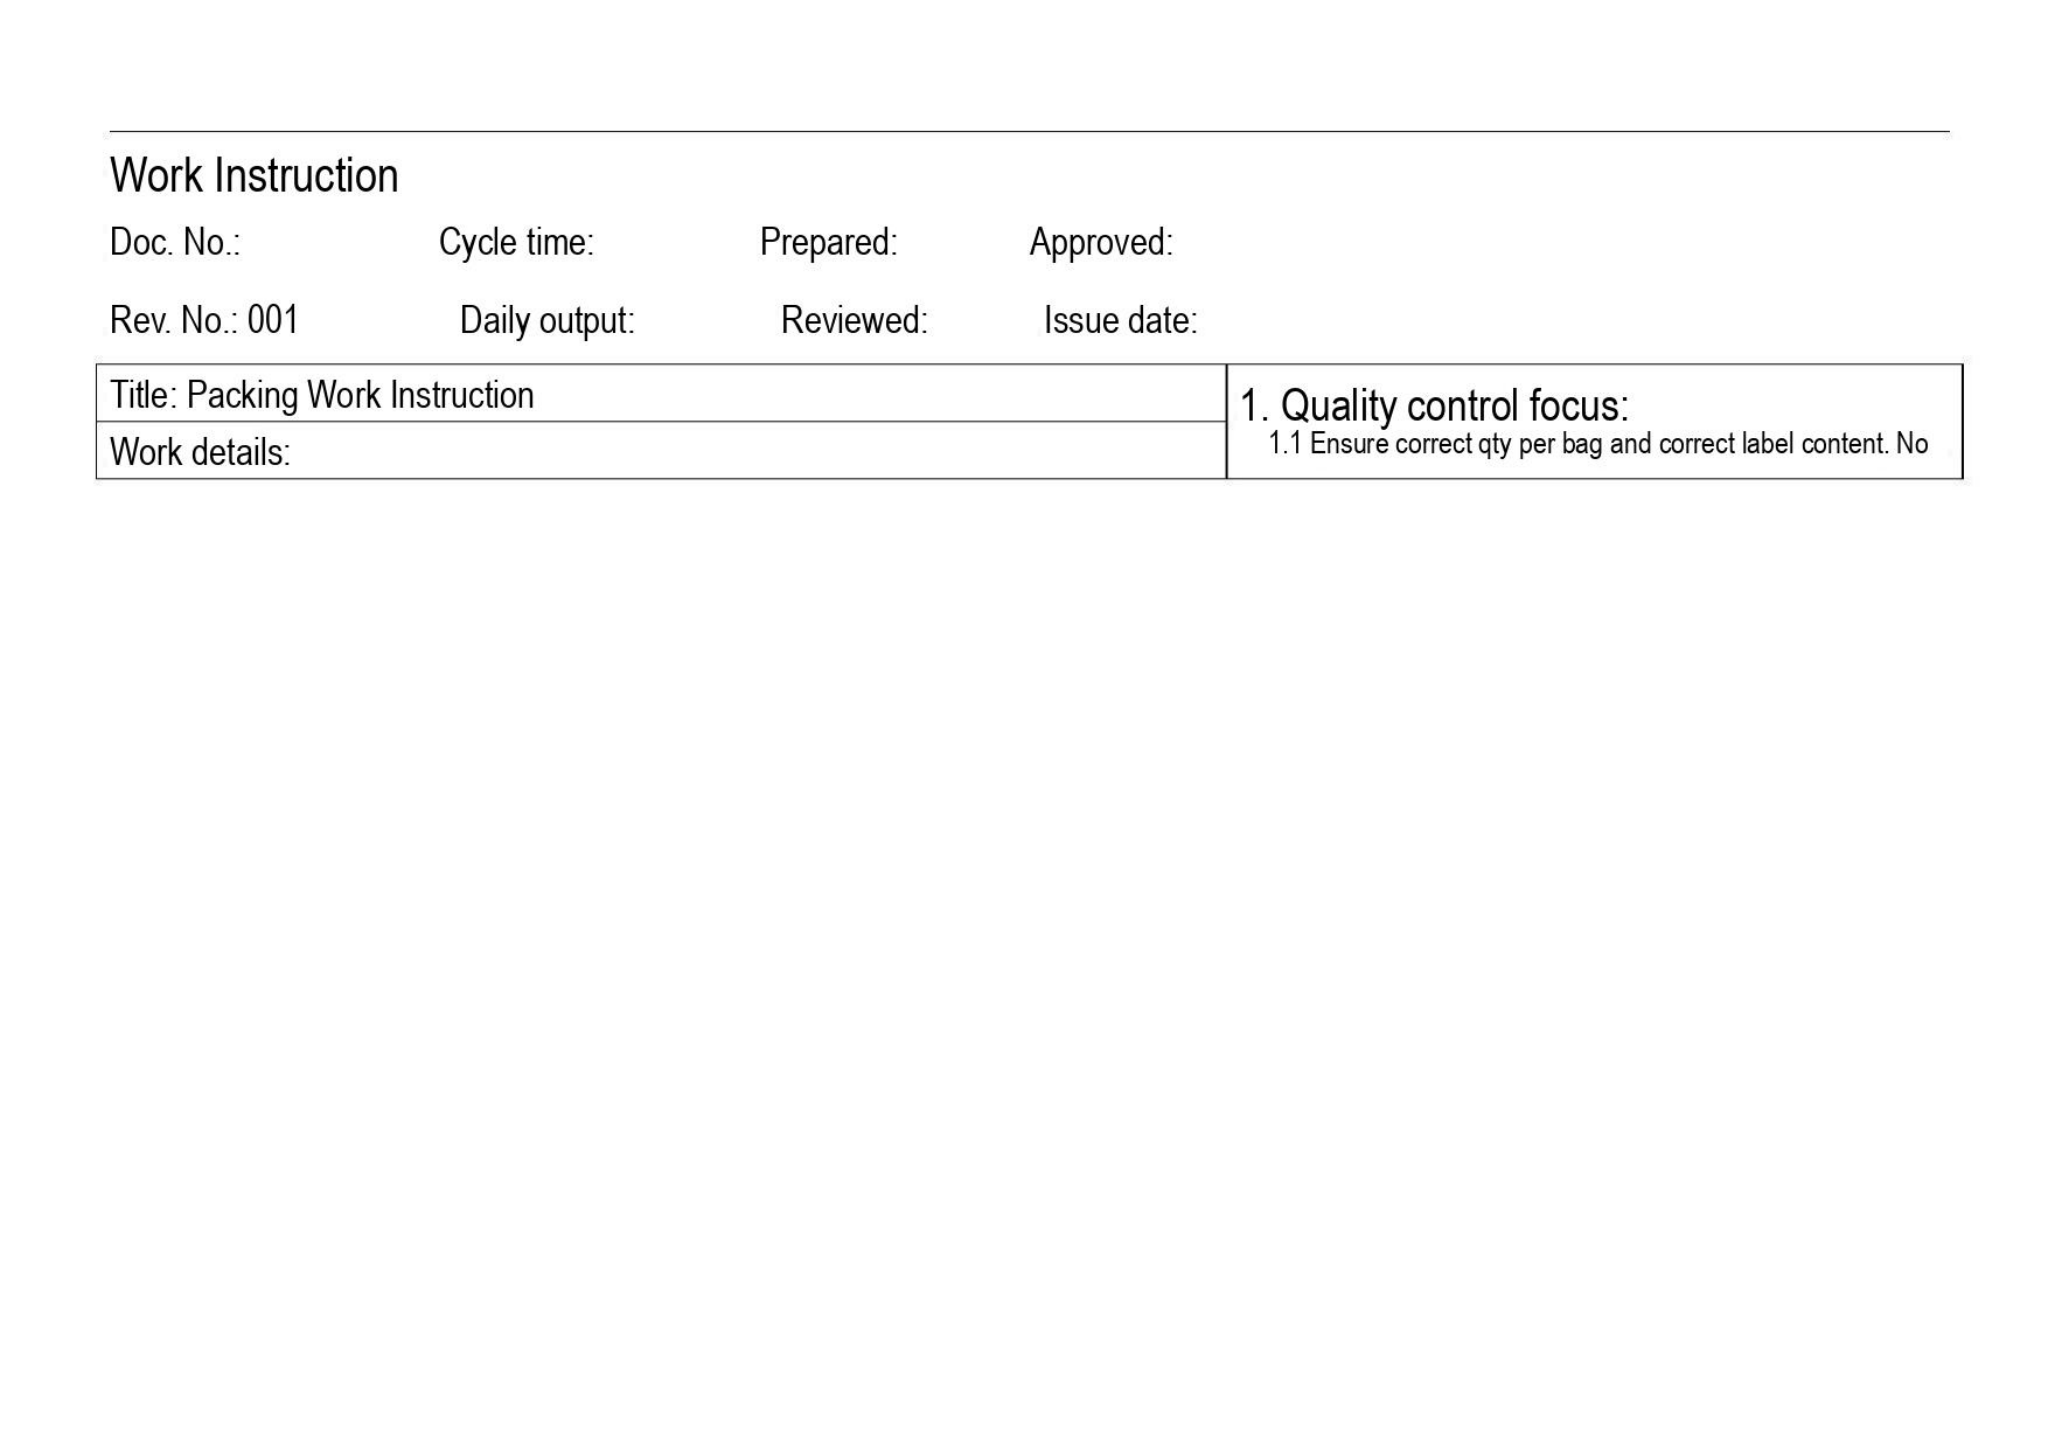Work Instruction

Doc. No.: Cycle time: Prepared: Approved:

Rev. No.: 001 Daily output: Reviewed: Issue date:

| Title: Packing Work Instruction | 1. Quality control focus: 1.1 Ensure correct qty per bag and correct label content. No |
|---|---|
| Work details: | |
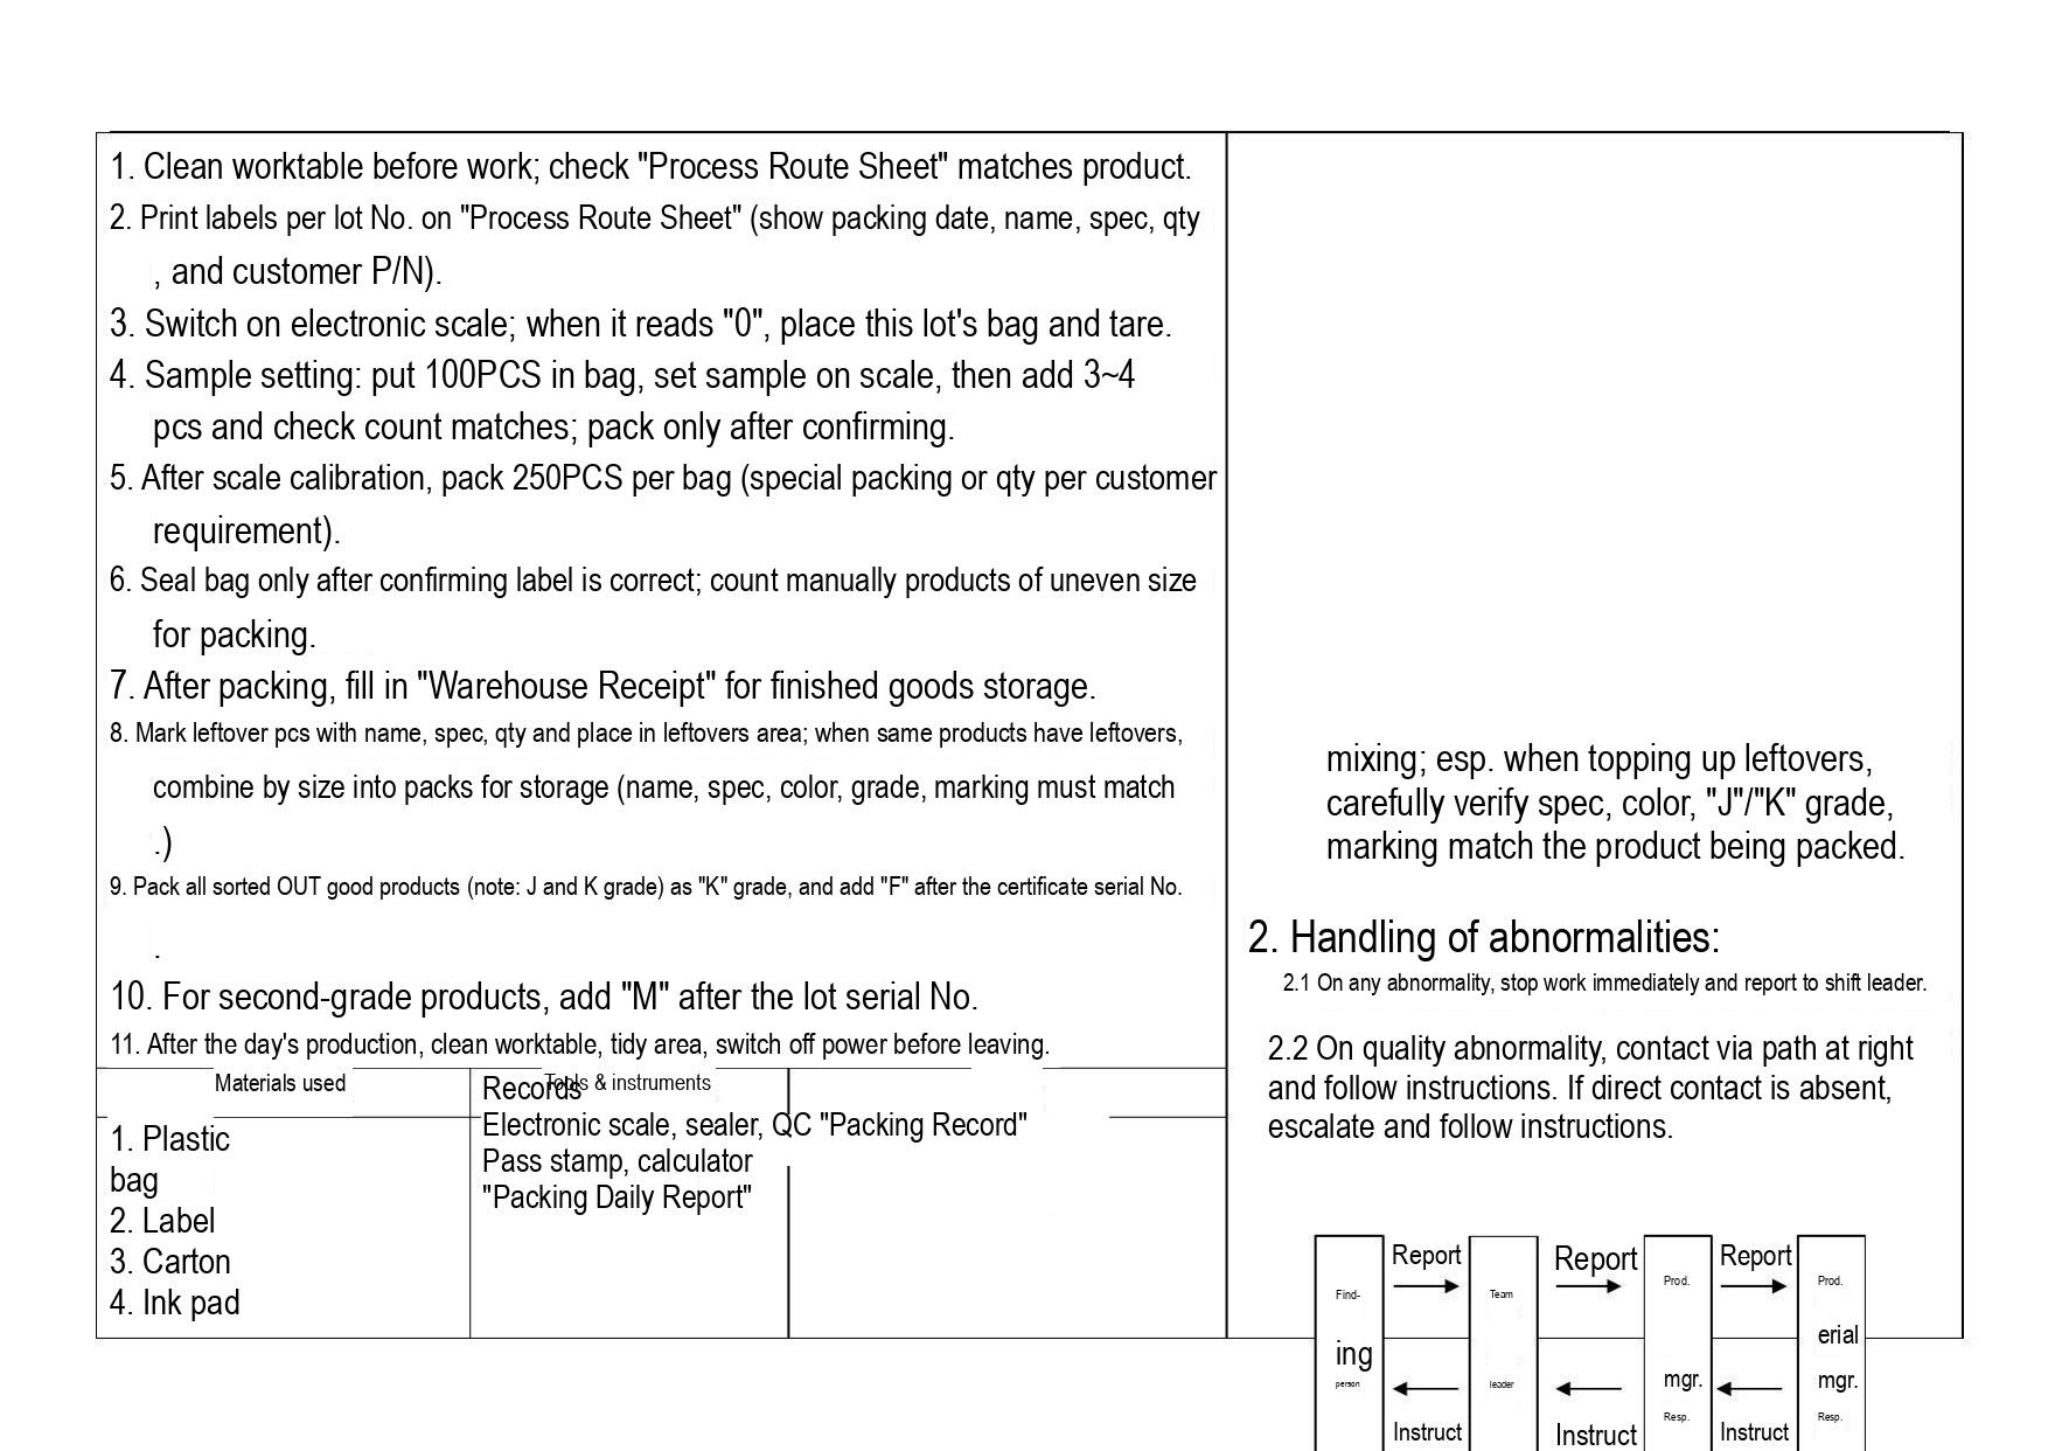1. Clean worktable before work; check "Process Route Sheet" matches product.
2. Print labels per lot No. on "Process Route Sheet" (show packing date, name, spec, qty, and customer P/N).
3. Switch on electronic scale; when it reads "0", place this lot's bag and tare.
4. Sample setting: put 100PCS in bag, set sample on scale, then add 3~4 pcs and check count matches; pack only after confirming.
5. After scale calibration, pack 250PCS per bag (special packing or qty per customer requirement).
6. Seal bag only after confirming label is correct; count manually products of uneven size for packing.
7. After packing, fill in "Warehouse Receipt" for finished goods storage.
8. Mark leftover pcs with name, spec, qty and place in leftovers area; when same products have leftovers, combine by size into packs for storage (name, spec, color, grade, marking must match.)
9. Pack all sorted OUT good products (note: J and K grade) as "K" grade, and add "F" after the certificate serial No.
10. For second-grade products, add "M" after the lot serial No.
11. After the day's production, clean worktable, tidy area, switch off power before leaving.

| Materials used | Records | Tools & instruments |
|---|---|---|
| 1. Plastic bag<br>2. Label<br>3. Carton<br>4. Ink pad | Electronic scale, sealer, QC "Packing Record"<br>Pass stamp, calculator<br>"Packing Daily Report" | |

mixing; esp. when topping up leftovers, carefully verify spec, color, "J"/"K" grade, marking match the product being packed.

2. Handling of abnormalities:
2.1 On any abnormality, stop work immediately and report to shift leader.
2.2 On quality abnormality, contact via path at right and follow instructions. If direct contact is absent, escalate and follow instructions.

Find-ing person
Report
Instruct
Team leader
Report
Instruct
Prod. mgr. Resp.
Report
Instruct
Prod. erial mgr. Resp.